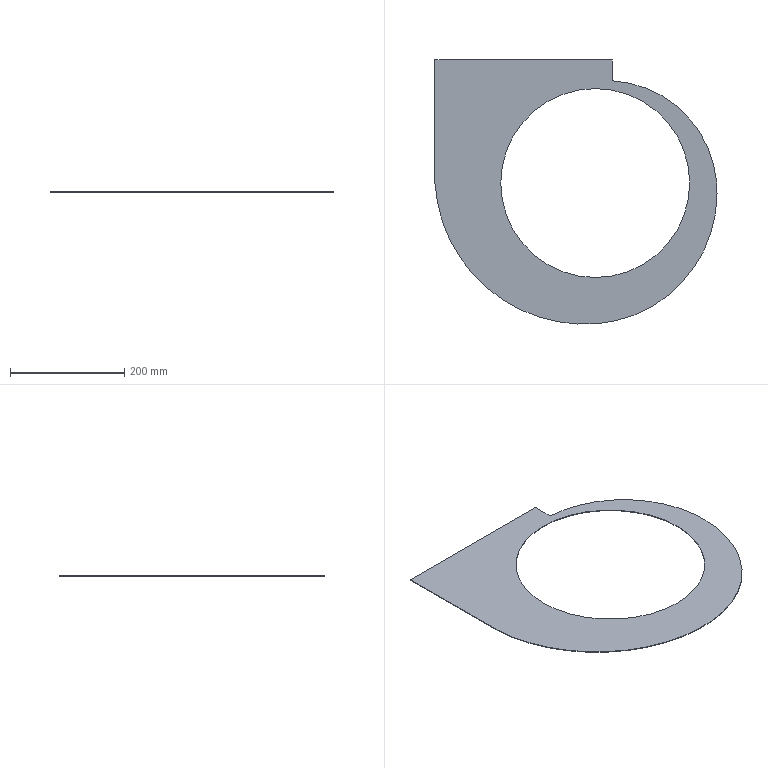Part | STEP file | HESS-408-70-15W-N-7-inner liner turbine panel | 1 solid | 11 faces | box 492.743 x 461.634 x 1 mm | volume 101400 mm3 | cylinder 6 | plane 5 | commonest cylinder face diameters 330 x2 456.243 x2 387.951 x1 524.472 x1
STEP:
#1=CARTESIAN_POINT('',(0.,0.,0.));
#2=DIRECTION('',(0.,0.,1.));
#3=DIRECTION('',(1.,0.,0.));
#4=AXIS2_PLACEMENT_3D('',#1,#2,#3);
#5=CARTESIAN_POINT('',(2081.954,652.923,-1.));
#6=VERTEX_POINT('',#5);
#7=CARTESIAN_POINT('',(2291.02,880.247,-1.));
#8=VERTEX_POINT('',#7);
#9=CARTESIAN_POINT('',(2062.898,880.247,-1.));
#10=DIRECTION('',(0.,0.,1.));
#11=DIRECTION('',(1.,0.,0.));
#12=AXIS2_PLACEMENT_3D('',#9,#10,#11);
#13=CIRCLE('',#12,228.121);
#14=CARTESIAN_POINT('',(2062.898,880.247,-1.));
#15=DIRECTION('',(0.,0.,1.));
#16=DIRECTION('',(1.,0.,0.));
#17=AXIS2_PLACEMENT_3D('',#14,#15,#16);
#18=CYLINDRICAL_SURFACE('',#17,228.121);
#19=CARTESIAN_POINT('',(0.,0.));
#20=DIRECTION('',(1.,0.));
#21=VECTOR('',#20,1.);
#22=LINE('',#19,#21);
#23=(GEOMETRIC_REPRESENTATION_CONTEXT(2)PARAMETRIC_REPRESENTATION_CONTEXT()REPRESENTATION_CONTEXT('',''));
#24=DEFINITIONAL_REPRESENTATION('',(#22),#23);
#25=PCURVE('',#18,#24);
#26=CARTESIAN_POINT('',(2062.898,880.247,-1.));
#27=DIRECTION('',(0.,0.,1.));
#28=DIRECTION('',(1.,0.,0.));
#29=AXIS2_PLACEMENT_3D('',#26,#27,#28);
#30=PLANE('',#29);
#31=CARTESIAN_POINT('',(0.,0.));
#32=DIRECTION('',(1.,0.));
#33=AXIS2_PLACEMENT_2D('',#31,#32);
#34=CIRCLE('',#33,228.121);
#35=(GEOMETRIC_REPRESENTATION_CONTEXT(2)PARAMETRIC_REPRESENTATION_CONTEXT()REPRESENTATION_CONTEXT('',''));
#36=DEFINITIONAL_REPRESENTATION('',(#34),#35);
#37=PCURVE('',#30,#36);
#38=SURFACE_CURVE('',#13,(#25,#37),.PCURVE_S1.);
#39=EDGE_CURVE('',#6,#8,#38,.T.);
#40=ORIENTED_EDGE('',*,*,#39,.T.);
#41=CARTESIAN_POINT('',(2291.02,880.247,0.));
#42=VERTEX_POINT('',#41);
#43=CARTESIAN_POINT('',(2291.02,880.247,-1.));
#44=DIRECTION('',(0.,0.,1.));
#45=VECTOR('',#44,1.);
#46=LINE('',#43,#45);
#47=CARTESIAN_POINT('',(6.283,0.));
#48=DIRECTION('',(0.,1.));
#49=VECTOR('',#48,1.);
#50=LINE('',#47,#49);
#51=(GEOMETRIC_REPRESENTATION_CONTEXT(2)PARAMETRIC_REPRESENTATION_CONTEXT()REPRESENTATION_CONTEXT('',''));
#52=DEFINITIONAL_REPRESENTATION('',(#50),#51);
#53=PCURVE('',#18,#52);
#54=CARTESIAN_POINT('',(2062.898,880.247,-1.));
#55=DIRECTION('',(0.,0.,1.));
#56=DIRECTION('',(1.,0.,0.));
#57=AXIS2_PLACEMENT_3D('',#54,#55,#56);
#58=CYLINDRICAL_SURFACE('',#57,228.121);
#59=CARTESIAN_POINT('',(0.,0.));
#60=DIRECTION('',(0.,1.));
#61=VECTOR('',#60,1.);
#62=LINE('',#59,#61);
#63=(GEOMETRIC_REPRESENTATION_CONTEXT(2)PARAMETRIC_REPRESENTATION_CONTEXT()REPRESENTATION_CONTEXT('',''));
#64=DEFINITIONAL_REPRESENTATION('',(#62),#63);
#65=PCURVE('',#58,#64);
#66=SURFACE_CURVE('',#46,(#53,#65),.PCURVE_S1.);
#67=EDGE_CURVE('',#8,#42,#66,.T.);
#68=ORIENTED_EDGE('',*,*,#67,.T.);
#69=CARTESIAN_POINT('',(2081.954,652.923,0.));
#70=VERTEX_POINT('',#69);
#71=CARTESIAN_POINT('',(2062.898,880.247,0.));
#72=DIRECTION('',(0.,0.,1.));
#73=DIRECTION('',(1.,0.,0.));
#74=AXIS2_PLACEMENT_3D('',#71,#72,#73);
#75=CIRCLE('',#74,228.121);
#76=CARTESIAN_POINT('',(0.,1.));
#77=DIRECTION('',(1.,0.));
#78=VECTOR('',#77,1.);
#79=LINE('',#76,#78);
#80=(GEOMETRIC_REPRESENTATION_CONTEXT(2)PARAMETRIC_REPRESENTATION_CONTEXT()REPRESENTATION_CONTEXT('',''));
#81=DEFINITIONAL_REPRESENTATION('',(#79),#80);
#82=PCURVE('',#18,#81);
#83=CARTESIAN_POINT('',(2062.898,880.247,0.));
#84=DIRECTION('',(0.,0.,1.));
#85=DIRECTION('',(1.,0.,0.));
#86=AXIS2_PLACEMENT_3D('',#83,#84,#85);
#87=PLANE('',#86);
#88=CARTESIAN_POINT('',(0.,0.));
#89=DIRECTION('',(1.,0.));
#90=AXIS2_PLACEMENT_2D('',#88,#89);
#91=CIRCLE('',#90,228.121);
#92=(GEOMETRIC_REPRESENTATION_CONTEXT(2)PARAMETRIC_REPRESENTATION_CONTEXT()REPRESENTATION_CONTEXT('',''));
#93=DEFINITIONAL_REPRESENTATION('',(#91),#92);
#94=PCURVE('',#87,#93);
#95=SURFACE_CURVE('',#75,(#82,#94),.PCURVE_S1.);
#96=EDGE_CURVE('',#70,#42,#95,.T.);
#97=ORIENTED_EDGE('',*,*,#96,.F.);
#98=CARTESIAN_POINT('',(2081.954,652.923,-1.));
#99=DIRECTION('',(0.,0.,1.));
#100=VECTOR('',#99,1.);
#101=LINE('',#98,#100);
#102=CARTESIAN_POINT('',(4.796,0.));
#103=DIRECTION('',(0.,1.));
#104=VECTOR('',#103,1.);
#105=LINE('',#102,#104);
#106=(GEOMETRIC_REPRESENTATION_CONTEXT(2)PARAMETRIC_REPRESENTATION_CONTEXT()REPRESENTATION_CONTEXT('',''));
#107=DEFINITIONAL_REPRESENTATION('',(#105),#106);
#108=PCURVE('',#18,#107);
#109=CARTESIAN_POINT('',(2060.048,914.242,-1.));
#110=DIRECTION('',(0.,0.,1.));
#111=DIRECTION('',(1.,0.,0.));
#112=AXIS2_PLACEMENT_3D('',#109,#110,#111);
#113=CYLINDRICAL_SURFACE('',#112,262.236);
#114=CARTESIAN_POINT('',(4.796,0.));
#115=DIRECTION('',(0.,1.));
#116=VECTOR('',#115,1.);
#117=LINE('',#114,#116);
#118=(GEOMETRIC_REPRESENTATION_CONTEXT(2)PARAMETRIC_REPRESENTATION_CONTEXT()REPRESENTATION_CONTEXT('',''));
#119=DEFINITIONAL_REPRESENTATION('',(#117),#118);
#120=PCURVE('',#113,#119);
#121=SURFACE_CURVE('',#101,(#108,#120),.PCURVE_S1.);
#122=EDGE_CURVE('',#6,#70,#121,.T.);
#123=ORIENTED_EDGE('',*,*,#122,.F.);
#124=EDGE_LOOP('',(#40,#68,#97,#123));
#125=FACE_BOUND('',#124,.T.);
#126=ADVANCED_FACE('',(#125),#18,.T.);
#127=CARTESIAN_POINT('',(2243.277,898.641,-1.));
#128=VERTEX_POINT('',#127);
#129=CARTESIAN_POINT('',(2243.277,898.641,0.));
#130=VERTEX_POINT('',#129);
#131=CARTESIAN_POINT('',(2243.277,898.641,-1.));
#132=DIRECTION('',(0.,0.,1.));
#133=VECTOR('',#132,1.);
#134=LINE('',#131,#133);
#135=CARTESIAN_POINT('',(2078.277,898.641,-1.));
#136=DIRECTION('',(0.,0.,1.));
#137=DIRECTION('',(1.,0.,0.));
#138=AXIS2_PLACEMENT_3D('',#135,#136,#137);
#139=CYLINDRICAL_SURFACE('',#138,165.);
#140=CARTESIAN_POINT('',(6.283,0.));
#141=DIRECTION('',(0.,1.));
#142=VECTOR('',#141,1.);
#143=LINE('',#140,#142);
#144=(GEOMETRIC_REPRESENTATION_CONTEXT(2)PARAMETRIC_REPRESENTATION_CONTEXT()REPRESENTATION_CONTEXT('',''));
#145=DEFINITIONAL_REPRESENTATION('',(#143),#144);
#146=PCURVE('',#139,#145);
#147=CARTESIAN_POINT('',(2078.277,898.641,-1.));
#148=DIRECTION('',(0.,0.,1.));
#149=DIRECTION('',(1.,0.,0.));
#150=AXIS2_PLACEMENT_3D('',#147,#148,#149);
#151=CYLINDRICAL_SURFACE('',#150,165.);
#152=CARTESIAN_POINT('',(0.,0.));
#153=DIRECTION('',(0.,1.));
#154=VECTOR('',#153,1.);
#155=LINE('',#152,#154);
#156=(GEOMETRIC_REPRESENTATION_CONTEXT(2)PARAMETRIC_REPRESENTATION_CONTEXT()REPRESENTATION_CONTEXT('',''));
#157=DEFINITIONAL_REPRESENTATION('',(#155),#156);
#158=PCURVE('',#151,#157);
#159=SURFACE_CURVE('',#134,(#146,#158),.PCURVE_S1.);
#160=EDGE_CURVE('',#128,#130,#159,.T.);
#161=ORIENTED_EDGE('',*,*,#160,.T.);
#162=CARTESIAN_POINT('',(1913.277,898.641,0.));
#163=VERTEX_POINT('',#162);
#164=CARTESIAN_POINT('',(2078.277,898.641,0.));
#165=DIRECTION('',(0.,0.,-1.));
#166=DIRECTION('',(1.,0.,0.));
#167=AXIS2_PLACEMENT_3D('',#164,#165,#166);
#168=CIRCLE('',#167,165.);
#169=CARTESIAN_POINT('',(6.283,1.));
#170=DIRECTION('',(-1.,0.));
#171=VECTOR('',#170,1.);
#172=LINE('',#169,#171);
#173=(GEOMETRIC_REPRESENTATION_CONTEXT(2)PARAMETRIC_REPRESENTATION_CONTEXT()REPRESENTATION_CONTEXT('',''));
#174=DEFINITIONAL_REPRESENTATION('',(#172),#173);
#175=PCURVE('',#139,#174);
#176=CARTESIAN_POINT('',(180.379,18.394));
#177=CARTESIAN_POINT('',(180.379,-267.395));
#178=CARTESIAN_POINT('',(-67.121,-124.5));
#179=CARTESIAN_POINT('',(-314.621,18.394));
#180=CARTESIAN_POINT('',(-67.121,161.288));
#181=CARTESIAN_POINT('',(180.379,304.182));
#182=CARTESIAN_POINT('',(180.379,18.394));
#183=(BOUNDED_CURVE()B_SPLINE_CURVE(2,(#176,#177,#178,#179,#180,#181,#182),.UNSPECIFIED.,.T.,.F.)B_SPLINE_CURVE_WITH_KNOTS((1,2,2,2,2,1),(-2.094,0.,2.094,4.189,6.283,8.378),.UNSPECIFIED.)CURVE()GEOMETRIC_REPRESENTATION_ITEM()RATIONAL_B_SPLINE_CURVE((1.,0.5,1.,0.5,1.,0.5,1.))REPRESENTATION_ITEM(''));
#184=(GEOMETRIC_REPRESENTATION_CONTEXT(2)PARAMETRIC_REPRESENTATION_CONTEXT()REPRESENTATION_CONTEXT('',''));
#185=DEFINITIONAL_REPRESENTATION('',(#183),#184);
#186=PCURVE('',#87,#185);
#187=SURFACE_CURVE('',#168,(#175,#186),.PCURVE_S1.);
#188=EDGE_CURVE('',#130,#163,#187,.T.);
#189=ORIENTED_EDGE('',*,*,#188,.T.);
#190=CARTESIAN_POINT('',(1913.277,898.641,-1.));
#191=VERTEX_POINT('',#190);
#192=CARTESIAN_POINT('',(1913.277,898.641,-1.));
#193=DIRECTION('',(0.,0.,1.));
#194=VECTOR('',#193,1.);
#195=LINE('',#192,#194);
#196=CARTESIAN_POINT('',(3.142,0.));
#197=DIRECTION('',(0.,1.));
#198=VECTOR('',#197,1.);
#199=LINE('',#196,#198);
#200=(GEOMETRIC_REPRESENTATION_CONTEXT(2)PARAMETRIC_REPRESENTATION_CONTEXT()REPRESENTATION_CONTEXT('',''));
#201=DEFINITIONAL_REPRESENTATION('',(#199),#200);
#202=PCURVE('',#139,#201);
#203=CARTESIAN_POINT('',(3.142,0.));
#204=DIRECTION('',(0.,1.));
#205=VECTOR('',#204,1.);
#206=LINE('',#203,#205);
#207=(GEOMETRIC_REPRESENTATION_CONTEXT(2)PARAMETRIC_REPRESENTATION_CONTEXT()REPRESENTATION_CONTEXT('',''));
#208=DEFINITIONAL_REPRESENTATION('',(#206),#207);
#209=PCURVE('',#151,#208);
#210=SURFACE_CURVE('',#195,(#202,#209),.PCURVE_S1.);
#211=EDGE_CURVE('',#191,#163,#210,.T.);
#212=ORIENTED_EDGE('',*,*,#211,.F.);
#213=CARTESIAN_POINT('',(2078.277,898.641,-1.));
#214=DIRECTION('',(0.,0.,1.));
#215=DIRECTION('',(1.,0.,0.));
#216=AXIS2_PLACEMENT_3D('',#213,#214,#215);
#217=CIRCLE('',#216,165.);
#218=CARTESIAN_POINT('',(0.,0.));
#219=DIRECTION('',(1.,0.));
#220=VECTOR('',#219,1.);
#221=LINE('',#218,#220);
#222=(GEOMETRIC_REPRESENTATION_CONTEXT(2)PARAMETRIC_REPRESENTATION_CONTEXT()REPRESENTATION_CONTEXT('',''));
#223=DEFINITIONAL_REPRESENTATION('',(#221),#222);
#224=PCURVE('',#139,#223);
#225=CARTESIAN_POINT('',(15.379,18.394));
#226=DIRECTION('',(1.,0.));
#227=AXIS2_PLACEMENT_2D('',#225,#226);
#228=CIRCLE('',#227,165.);
#229=(GEOMETRIC_REPRESENTATION_CONTEXT(2)PARAMETRIC_REPRESENTATION_CONTEXT()REPRESENTATION_CONTEXT('',''));
#230=DEFINITIONAL_REPRESENTATION('',(#228),#229);
#231=PCURVE('',#30,#230);
#232=SURFACE_CURVE('',#217,(#224,#231),.PCURVE_S1.);
#233=EDGE_CURVE('',#191,#128,#232,.T.);
#234=ORIENTED_EDGE('',*,*,#233,.T.);
#235=EDGE_LOOP('',(#161,#189,#212,#234));
#236=FACE_BOUND('',#235,.F.);
#237=ADVANCED_FACE('',(#236),#139,.F.);
#238=CARTESIAN_POINT('',(1798.277,1113.641,0.));
#239=VERTEX_POINT('',#238);
#240=CARTESIAN_POINT('',(1798.277,898.641,0.));
#241=VERTEX_POINT('',#240);
#242=CARTESIAN_POINT('',(1798.277,880.247,0.));
#243=DIRECTION('',(0.,-1.,0.));
#244=VECTOR('',#243,1.);
#245=LINE('',#242,#244);
#246=CARTESIAN_POINT('',(-264.621,0.));
#247=DIRECTION('',(0.,-1.));
#248=VECTOR('',#247,1.);
#249=LINE('',#246,#248);
#250=(GEOMETRIC_REPRESENTATION_CONTEXT(2)PARAMETRIC_REPRESENTATION_CONTEXT()REPRESENTATION_CONTEXT('',''));
#251=DEFINITIONAL_REPRESENTATION('',(#249),#250);
#252=PCURVE('',#87,#251);
#253=CARTESIAN_POINT('',(1798.277,898.641,-1.));
#254=DIRECTION('',(-1.,0.,0.));
#255=DIRECTION('',(0.,-1.,0.));
#256=AXIS2_PLACEMENT_3D('',#253,#254,#255);
#257=PLANE('',#256);
#258=CARTESIAN_POINT('',(18.394,1.));
#259=DIRECTION('',(1.,0.));
#260=VECTOR('',#259,1.);
#261=LINE('',#258,#260);
#262=(GEOMETRIC_REPRESENTATION_CONTEXT(2)PARAMETRIC_REPRESENTATION_CONTEXT()REPRESENTATION_CONTEXT('',''));
#263=DEFINITIONAL_REPRESENTATION('',(#261),#262);
#264=PCURVE('',#257,#263);
#265=SURFACE_CURVE('',#245,(#252,#264),.PCURVE_S1.);
#266=EDGE_CURVE('',#239,#241,#265,.T.);
#267=ORIENTED_EDGE('',*,*,#266,.T.);
#268=CARTESIAN_POINT('',(2060.048,914.242,0.));
#269=DIRECTION('',(0.,0.,1.));
#270=DIRECTION('',(1.,0.,0.));
#271=AXIS2_PLACEMENT_3D('',#268,#269,#270);
#272=CIRCLE('',#271,262.236);
#273=CARTESIAN_POINT('',(-2.85,33.996));
#274=DIRECTION('',(1.,0.));
#275=AXIS2_PLACEMENT_2D('',#273,#274);
#276=CIRCLE('',#275,262.236);
#277=(GEOMETRIC_REPRESENTATION_CONTEXT(2)PARAMETRIC_REPRESENTATION_CONTEXT()REPRESENTATION_CONTEXT('',''));
#278=DEFINITIONAL_REPRESENTATION('',(#276),#277);
#279=PCURVE('',#87,#278);
#280=CARTESIAN_POINT('',(0.,1.));
#281=DIRECTION('',(1.,0.));
#282=VECTOR('',#281,1.);
#283=LINE('',#280,#282);
#284=(GEOMETRIC_REPRESENTATION_CONTEXT(2)PARAMETRIC_REPRESENTATION_CONTEXT()REPRESENTATION_CONTEXT('',''));
#285=DEFINITIONAL_REPRESENTATION('',(#283),#284);
#286=PCURVE('',#113,#285);
#287=SURFACE_CURVE('',#272,(#279,#286),.PCURVE_S1.);
#288=EDGE_CURVE('',#241,#70,#287,.T.);
#289=ORIENTED_EDGE('',*,*,#288,.T.);
#290=ORIENTED_EDGE('',*,*,#96,.T.);
#291=CARTESIAN_POINT('',(2289.943,902.379,0.));
#292=VERTEX_POINT('',#291);
#293=CARTESIAN_POINT('',(2062.898,880.247,0.));
#294=DIRECTION('',(0.,0.,1.));
#295=DIRECTION('',(1.,0.,0.));
#296=AXIS2_PLACEMENT_3D('',#293,#294,#295);
#297=CIRCLE('',#296,228.121);
#298=CARTESIAN_POINT('',(0.,0.));
#299=DIRECTION('',(1.,0.));
#300=AXIS2_PLACEMENT_2D('',#298,#299);
#301=CIRCLE('',#300,228.121);
#302=(GEOMETRIC_REPRESENTATION_CONTEXT(2)PARAMETRIC_REPRESENTATION_CONTEXT()REPRESENTATION_CONTEXT('',''));
#303=DEFINITIONAL_REPRESENTATION('',(#301),#302);
#304=PCURVE('',#87,#303);
#305=CARTESIAN_POINT('',(0.,1.));
#306=DIRECTION('',(1.,0.));
#307=VECTOR('',#306,1.);
#308=LINE('',#305,#307);
#309=(GEOMETRIC_REPRESENTATION_CONTEXT(2)PARAMETRIC_REPRESENTATION_CONTEXT()REPRESENTATION_CONTEXT('',''));
#310=DEFINITIONAL_REPRESENTATION('',(#308),#309);
#311=PCURVE('',#58,#310);
#312=SURFACE_CURVE('',#297,(#304,#311),.PCURVE_S1.);
#313=EDGE_CURVE('',#42,#292,#312,.T.);
#314=ORIENTED_EDGE('',*,*,#313,.T.);
#315=CARTESIAN_POINT('',(2108.277,1077.2,0.));
#316=VERTEX_POINT('',#315);
#317=CARTESIAN_POINT('',(2096.883,883.56,0.));
#318=DIRECTION('',(0.,0.,1.));
#319=DIRECTION('',(1.,0.,0.));
#320=AXIS2_PLACEMENT_3D('',#317,#318,#319);
#321=CIRCLE('',#320,193.975);
#322=CARTESIAN_POINT('',(33.985,3.313));
#323=DIRECTION('',(1.,0.));
#324=AXIS2_PLACEMENT_2D('',#322,#323);
#325=CIRCLE('',#324,193.975);
#326=(GEOMETRIC_REPRESENTATION_CONTEXT(2)PARAMETRIC_REPRESENTATION_CONTEXT()REPRESENTATION_CONTEXT('',''));
#327=DEFINITIONAL_REPRESENTATION('',(#325),#326);
#328=PCURVE('',#87,#327);
#329=CARTESIAN_POINT('',(2096.883,883.56,-1.));
#330=DIRECTION('',(0.,0.,1.));
#331=DIRECTION('',(1.,0.,0.));
#332=AXIS2_PLACEMENT_3D('',#329,#330,#331);
#333=CYLINDRICAL_SURFACE('',#332,193.975);
#334=CARTESIAN_POINT('',(0.,1.));
#335=DIRECTION('',(1.,0.));
#336=VECTOR('',#335,1.);
#337=LINE('',#334,#336);
#338=(GEOMETRIC_REPRESENTATION_CONTEXT(2)PARAMETRIC_REPRESENTATION_CONTEXT()REPRESENTATION_CONTEXT('',''));
#339=DEFINITIONAL_REPRESENTATION('',(#337),#338);
#340=PCURVE('',#333,#339);
#341=SURFACE_CURVE('',#321,(#328,#340),.PCURVE_S1.);
#342=EDGE_CURVE('',#292,#316,#341,.T.);
#343=ORIENTED_EDGE('',*,*,#342,.T.);
#344=CARTESIAN_POINT('',(2108.277,1113.641,0.));
#345=VERTEX_POINT('',#344);
#346=CARTESIAN_POINT('',(2108.277,880.247,0.));
#347=DIRECTION('',(0.,1.,0.));
#348=VECTOR('',#347,1.);
#349=LINE('',#346,#348);
#350=CARTESIAN_POINT('',(45.379,0.));
#351=DIRECTION('',(0.,1.));
#352=VECTOR('',#351,1.);
#353=LINE('',#350,#352);
#354=(GEOMETRIC_REPRESENTATION_CONTEXT(2)PARAMETRIC_REPRESENTATION_CONTEXT()REPRESENTATION_CONTEXT('',''));
#355=DEFINITIONAL_REPRESENTATION('',(#353),#354);
#356=PCURVE('',#87,#355);
#357=CARTESIAN_POINT('',(2108.277,1113.641,-1.));
#358=DIRECTION('',(1.,0.,0.));
#359=DIRECTION('',(0.,0.,-1.));
#360=AXIS2_PLACEMENT_3D('',#357,#358,#359);
#361=PLANE('',#360);
#362=CARTESIAN_POINT('',(-1.,-233.394));
#363=DIRECTION('',(0.,1.));
#364=VECTOR('',#363,1.);
#365=LINE('',#362,#364);
#366=(GEOMETRIC_REPRESENTATION_CONTEXT(2)PARAMETRIC_REPRESENTATION_CONTEXT()REPRESENTATION_CONTEXT('',''));
#367=DEFINITIONAL_REPRESENTATION('',(#365),#366);
#368=PCURVE('',#361,#367);
#369=SURFACE_CURVE('',#349,(#356,#368),.PCURVE_S1.);
#370=EDGE_CURVE('',#316,#345,#369,.T.);
#371=ORIENTED_EDGE('',*,*,#370,.T.);
#372=CARTESIAN_POINT('',(2062.898,1113.641,0.));
#373=DIRECTION('',(-1.,0.,0.));
#374=VECTOR('',#373,1.);
#375=LINE('',#372,#374);
#376=CARTESIAN_POINT('',(0.,233.394));
#377=DIRECTION('',(-1.,0.));
#378=VECTOR('',#377,1.);
#379=LINE('',#376,#378);
#380=(GEOMETRIC_REPRESENTATION_CONTEXT(2)PARAMETRIC_REPRESENTATION_CONTEXT()REPRESENTATION_CONTEXT('',''));
#381=DEFINITIONAL_REPRESENTATION('',(#379),#380);
#382=PCURVE('',#87,#381);
#383=CARTESIAN_POINT('',(2108.277,1113.641,-1.));
#384=DIRECTION('',(0.,1.,0.));
#385=DIRECTION('',(0.,0.,1.));
#386=AXIS2_PLACEMENT_3D('',#383,#384,#385);
#387=PLANE('',#386);
#388=CARTESIAN_POINT('',(1.,-45.379));
#389=DIRECTION('',(0.,-1.));
#390=VECTOR('',#389,1.);
#391=LINE('',#388,#390);
#392=(GEOMETRIC_REPRESENTATION_CONTEXT(2)PARAMETRIC_REPRESENTATION_CONTEXT()REPRESENTATION_CONTEXT('',''));
#393=DEFINITIONAL_REPRESENTATION('',(#391),#392);
#394=PCURVE('',#387,#393);
#395=SURFACE_CURVE('',#375,(#382,#394),.PCURVE_S1.);
#396=EDGE_CURVE('',#345,#239,#395,.T.);
#397=ORIENTED_EDGE('',*,*,#396,.T.);
#398=EDGE_LOOP('',(#267,#289,#290,#314,#343,#371,#397));
#399=FACE_BOUND('',#398,.T.);
#400=ORIENTED_EDGE('',*,*,#188,.T.);
#401=CARTESIAN_POINT('',(2078.277,898.641,0.));
#402=DIRECTION('',(0.,0.,-1.));
#403=DIRECTION('',(1.,0.,0.));
#404=AXIS2_PLACEMENT_3D('',#401,#402,#403);
#405=CIRCLE('',#404,165.);
#406=CARTESIAN_POINT('',(180.379,18.394));
#407=CARTESIAN_POINT('',(180.379,-267.395));
#408=CARTESIAN_POINT('',(-67.121,-124.5));
#409=CARTESIAN_POINT('',(-314.621,18.394));
#410=CARTESIAN_POINT('',(-67.121,161.288));
#411=CARTESIAN_POINT('',(180.379,304.182));
#412=CARTESIAN_POINT('',(180.379,18.394));
#413=(BOUNDED_CURVE()B_SPLINE_CURVE(2,(#406,#407,#408,#409,#410,#411,#412),.UNSPECIFIED.,.T.,.F.)B_SPLINE_CURVE_WITH_KNOTS((1,2,2,2,2,1),(-2.094,0.,2.094,4.189,6.283,8.378),.UNSPECIFIED.)CURVE()GEOMETRIC_REPRESENTATION_ITEM()RATIONAL_B_SPLINE_CURVE((1.,0.5,1.,0.5,1.,0.5,1.))REPRESENTATION_ITEM(''));
#414=(GEOMETRIC_REPRESENTATION_CONTEXT(2)PARAMETRIC_REPRESENTATION_CONTEXT()REPRESENTATION_CONTEXT('',''));
#415=DEFINITIONAL_REPRESENTATION('',(#413),#414);
#416=PCURVE('',#87,#415);
#417=CARTESIAN_POINT('',(6.283,1.));
#418=DIRECTION('',(-1.,0.));
#419=VECTOR('',#418,1.);
#420=LINE('',#417,#419);
#421=(GEOMETRIC_REPRESENTATION_CONTEXT(2)PARAMETRIC_REPRESENTATION_CONTEXT()REPRESENTATION_CONTEXT('',''));
#422=DEFINITIONAL_REPRESENTATION('',(#420),#421);
#423=PCURVE('',#151,#422);
#424=SURFACE_CURVE('',#405,(#416,#423),.PCURVE_S1.);
#425=EDGE_CURVE('',#163,#130,#424,.T.);
#426=ORIENTED_EDGE('',*,*,#425,.T.);
#427=EDGE_LOOP('',(#400,#426));
#428=FACE_BOUND('',#427,.T.);
#429=ADVANCED_FACE('',(#399,#428),#87,.T.);
#430=CARTESIAN_POINT('',(1798.277,898.641,-1.));
#431=VERTEX_POINT('',#430);
#432=CARTESIAN_POINT('',(2060.048,914.242,-1.));
#433=DIRECTION('',(0.,0.,1.));
#434=DIRECTION('',(1.,0.,0.));
#435=AXIS2_PLACEMENT_3D('',#432,#433,#434);
#436=CIRCLE('',#435,262.236);
#437=CARTESIAN_POINT('',(0.,0.));
#438=DIRECTION('',(1.,0.));
#439=VECTOR('',#438,1.);
#440=LINE('',#437,#439);
#441=(GEOMETRIC_REPRESENTATION_CONTEXT(2)PARAMETRIC_REPRESENTATION_CONTEXT()REPRESENTATION_CONTEXT('',''));
#442=DEFINITIONAL_REPRESENTATION('',(#440),#441);
#443=PCURVE('',#113,#442);
#444=CARTESIAN_POINT('',(-2.85,33.996));
#445=DIRECTION('',(1.,0.));
#446=AXIS2_PLACEMENT_2D('',#444,#445);
#447=CIRCLE('',#446,262.236);
#448=(GEOMETRIC_REPRESENTATION_CONTEXT(2)PARAMETRIC_REPRESENTATION_CONTEXT()REPRESENTATION_CONTEXT('',''));
#449=DEFINITIONAL_REPRESENTATION('',(#447),#448);
#450=PCURVE('',#30,#449);
#451=SURFACE_CURVE('',#436,(#443,#450),.PCURVE_S1.);
#452=EDGE_CURVE('',#431,#6,#451,.T.);
#453=ORIENTED_EDGE('',*,*,#452,.T.);
#454=ORIENTED_EDGE('',*,*,#122,.T.);
#455=ORIENTED_EDGE('',*,*,#288,.F.);
#456=CARTESIAN_POINT('',(1798.277,898.641,-1.));
#457=DIRECTION('',(0.,0.,-1.));
#458=VECTOR('',#457,1.);
#459=LINE('',#456,#458);
#460=CARTESIAN_POINT('',(3.201,0.));
#461=DIRECTION('',(0.,-1.));
#462=VECTOR('',#461,1.);
#463=LINE('',#460,#462);
#464=(GEOMETRIC_REPRESENTATION_CONTEXT(2)PARAMETRIC_REPRESENTATION_CONTEXT()REPRESENTATION_CONTEXT('',''));
#465=DEFINITIONAL_REPRESENTATION('',(#463),#464);
#466=PCURVE('',#113,#465);
#467=CARTESIAN_POINT('',(0.,0.));
#468=DIRECTION('',(0.,-1.));
#469=VECTOR('',#468,1.);
#470=LINE('',#467,#469);
#471=(GEOMETRIC_REPRESENTATION_CONTEXT(2)PARAMETRIC_REPRESENTATION_CONTEXT()REPRESENTATION_CONTEXT('',''));
#472=DEFINITIONAL_REPRESENTATION('',(#470),#471);
#473=PCURVE('',#257,#472);
#474=SURFACE_CURVE('',#459,(#466,#473),.PCURVE_S1.);
#475=EDGE_CURVE('',#241,#431,#474,.T.);
#476=ORIENTED_EDGE('',*,*,#475,.T.);
#477=EDGE_LOOP('',(#453,#454,#455,#476));
#478=FACE_BOUND('',#477,.T.);
#479=ADVANCED_FACE('',(#478),#113,.T.);
#480=CARTESIAN_POINT('',(1798.277,1113.641,-1.));
#481=VERTEX_POINT('',#480);
#482=CARTESIAN_POINT('',(1798.277,898.641,-1.));
#483=DIRECTION('',(0.,-1.,0.));
#484=VECTOR('',#483,1.);
#485=LINE('',#482,#484);
#486=CARTESIAN_POINT('',(0.,0.));
#487=DIRECTION('',(1.,0.));
#488=VECTOR('',#487,1.);
#489=LINE('',#486,#488);
#490=(GEOMETRIC_REPRESENTATION_CONTEXT(2)PARAMETRIC_REPRESENTATION_CONTEXT()REPRESENTATION_CONTEXT('',''));
#491=DEFINITIONAL_REPRESENTATION('',(#489),#490);
#492=PCURVE('',#257,#491);
#493=CARTESIAN_POINT('',(-264.621,18.394));
#494=DIRECTION('',(0.,-1.));
#495=VECTOR('',#494,1.);
#496=LINE('',#493,#495);
#497=(GEOMETRIC_REPRESENTATION_CONTEXT(2)PARAMETRIC_REPRESENTATION_CONTEXT()REPRESENTATION_CONTEXT('',''));
#498=DEFINITIONAL_REPRESENTATION('',(#496),#497);
#499=PCURVE('',#30,#498);
#500=SURFACE_CURVE('',#485,(#492,#499),.PCURVE_S1.);
#501=EDGE_CURVE('',#481,#431,#500,.T.);
#502=ORIENTED_EDGE('',*,*,#501,.T.);
#503=ORIENTED_EDGE('',*,*,#475,.F.);
#504=ORIENTED_EDGE('',*,*,#266,.F.);
#505=CARTESIAN_POINT('',(1798.277,1113.641,-1.));
#506=DIRECTION('',(0.,0.,-1.));
#507=VECTOR('',#506,1.);
#508=LINE('',#505,#507);
#509=CARTESIAN_POINT('',(-215.,0.));
#510=DIRECTION('',(0.,-1.));
#511=VECTOR('',#510,1.);
#512=LINE('',#509,#511);
#513=(GEOMETRIC_REPRESENTATION_CONTEXT(2)PARAMETRIC_REPRESENTATION_CONTEXT()REPRESENTATION_CONTEXT('',''));
#514=DEFINITIONAL_REPRESENTATION('',(#512),#513);
#515=PCURVE('',#257,#514);
#516=CARTESIAN_POINT('',(0.,-310.));
#517=DIRECTION('',(-1.,0.));
#518=VECTOR('',#517,1.);
#519=LINE('',#516,#518);
#520=(GEOMETRIC_REPRESENTATION_CONTEXT(2)PARAMETRIC_REPRESENTATION_CONTEXT()REPRESENTATION_CONTEXT('',''));
#521=DEFINITIONAL_REPRESENTATION('',(#519),#520);
#522=PCURVE('',#387,#521);
#523=SURFACE_CURVE('',#508,(#515,#522),.PCURVE_S1.);
#524=EDGE_CURVE('',#239,#481,#523,.T.);
#525=ORIENTED_EDGE('',*,*,#524,.T.);
#526=EDGE_LOOP('',(#502,#503,#504,#525));
#527=FACE_BOUND('',#526,.T.);
#528=ADVANCED_FACE('',(#527),#257,.T.);
#529=CARTESIAN_POINT('',(2108.277,1113.641,-1.));
#530=VERTEX_POINT('',#529);
#531=CARTESIAN_POINT('',(2108.277,1113.641,-1.));
#532=DIRECTION('',(-1.,0.,0.));
#533=VECTOR('',#532,1.);
#534=LINE('',#531,#533);
#535=CARTESIAN_POINT('',(0.,0.));
#536=DIRECTION('',(0.,-1.));
#537=VECTOR('',#536,1.);
#538=LINE('',#535,#537);
#539=(GEOMETRIC_REPRESENTATION_CONTEXT(2)PARAMETRIC_REPRESENTATION_CONTEXT()REPRESENTATION_CONTEXT('',''));
#540=DEFINITIONAL_REPRESENTATION('',(#538),#539);
#541=PCURVE('',#387,#540);
#542=CARTESIAN_POINT('',(45.379,233.394));
#543=DIRECTION('',(-1.,0.));
#544=VECTOR('',#543,1.);
#545=LINE('',#542,#544);
#546=(GEOMETRIC_REPRESENTATION_CONTEXT(2)PARAMETRIC_REPRESENTATION_CONTEXT()REPRESENTATION_CONTEXT('',''));
#547=DEFINITIONAL_REPRESENTATION('',(#545),#546);
#548=PCURVE('',#30,#547);
#549=SURFACE_CURVE('',#534,(#541,#548),.PCURVE_S1.);
#550=EDGE_CURVE('',#530,#481,#549,.T.);
#551=ORIENTED_EDGE('',*,*,#550,.T.);
#552=ORIENTED_EDGE('',*,*,#524,.F.);
#553=ORIENTED_EDGE('',*,*,#396,.F.);
#554=CARTESIAN_POINT('',(2108.277,1113.641,-1.));
#555=DIRECTION('',(0.,0.,-1.));
#556=VECTOR('',#555,1.);
#557=LINE('',#554,#556);
#558=CARTESIAN_POINT('',(0.,0.));
#559=DIRECTION('',(-1.,0.));
#560=VECTOR('',#559,1.);
#561=LINE('',#558,#560);
#562=(GEOMETRIC_REPRESENTATION_CONTEXT(2)PARAMETRIC_REPRESENTATION_CONTEXT()REPRESENTATION_CONTEXT('',''));
#563=DEFINITIONAL_REPRESENTATION('',(#561),#562);
#564=PCURVE('',#387,#563);
#565=CARTESIAN_POINT('',(0.,0.));
#566=DIRECTION('',(1.,0.));
#567=VECTOR('',#566,1.);
#568=LINE('',#565,#567);
#569=(GEOMETRIC_REPRESENTATION_CONTEXT(2)PARAMETRIC_REPRESENTATION_CONTEXT()REPRESENTATION_CONTEXT('',''));
#570=DEFINITIONAL_REPRESENTATION('',(#568),#569);
#571=PCURVE('',#361,#570);
#572=SURFACE_CURVE('',#557,(#564,#571),.PCURVE_S1.);
#573=EDGE_CURVE('',#345,#530,#572,.T.);
#574=ORIENTED_EDGE('',*,*,#573,.T.);
#575=EDGE_LOOP('',(#551,#552,#553,#574));
#576=FACE_BOUND('',#575,.T.);
#577=ADVANCED_FACE('',(#576),#387,.T.);
#578=CARTESIAN_POINT('',(2108.277,1077.2,-1.));
#579=VERTEX_POINT('',#578);
#580=CARTESIAN_POINT('',(2108.277,1113.641,-1.));
#581=DIRECTION('',(0.,1.,0.));
#582=VECTOR('',#581,1.);
#583=LINE('',#580,#582);
#584=CARTESIAN_POINT('',(0.,0.));
#585=DIRECTION('',(0.,1.));
#586=VECTOR('',#585,1.);
#587=LINE('',#584,#586);
#588=(GEOMETRIC_REPRESENTATION_CONTEXT(2)PARAMETRIC_REPRESENTATION_CONTEXT()REPRESENTATION_CONTEXT('',''));
#589=DEFINITIONAL_REPRESENTATION('',(#587),#588);
#590=PCURVE('',#361,#589);
#591=CARTESIAN_POINT('',(45.379,233.394));
#592=DIRECTION('',(0.,1.));
#593=VECTOR('',#592,1.);
#594=LINE('',#591,#593);
#595=(GEOMETRIC_REPRESENTATION_CONTEXT(2)PARAMETRIC_REPRESENTATION_CONTEXT()REPRESENTATION_CONTEXT('',''));
#596=DEFINITIONAL_REPRESENTATION('',(#594),#595);
#597=PCURVE('',#30,#596);
#598=SURFACE_CURVE('',#583,(#590,#597),.PCURVE_S1.);
#599=EDGE_CURVE('',#579,#530,#598,.T.);
#600=ORIENTED_EDGE('',*,*,#599,.T.);
#601=ORIENTED_EDGE('',*,*,#573,.F.);
#602=ORIENTED_EDGE('',*,*,#370,.F.);
#603=CARTESIAN_POINT('',(2108.277,1077.2,-1.));
#604=DIRECTION('',(0.,0.,-1.));
#605=VECTOR('',#604,1.);
#606=LINE('',#603,#605);
#607=CARTESIAN_POINT('',(0.,-36.44));
#608=DIRECTION('',(1.,0.));
#609=VECTOR('',#608,1.);
#610=LINE('',#607,#609);
#611=(GEOMETRIC_REPRESENTATION_CONTEXT(2)PARAMETRIC_REPRESENTATION_CONTEXT()REPRESENTATION_CONTEXT('',''));
#612=DEFINITIONAL_REPRESENTATION('',(#610),#611);
#613=PCURVE('',#361,#612);
#614=CARTESIAN_POINT('',(1.512,0.));
#615=DIRECTION('',(0.,-1.));
#616=VECTOR('',#615,1.);
#617=LINE('',#614,#616);
#618=(GEOMETRIC_REPRESENTATION_CONTEXT(2)PARAMETRIC_REPRESENTATION_CONTEXT()REPRESENTATION_CONTEXT('',''));
#619=DEFINITIONAL_REPRESENTATION('',(#617),#618);
#620=PCURVE('',#333,#619);
#621=SURFACE_CURVE('',#606,(#613,#620),.PCURVE_S1.);
#622=EDGE_CURVE('',#316,#579,#621,.T.);
#623=ORIENTED_EDGE('',*,*,#622,.T.);
#624=EDGE_LOOP('',(#600,#601,#602,#623));
#625=FACE_BOUND('',#624,.T.);
#626=ADVANCED_FACE('',(#625),#361,.T.);
#627=CARTESIAN_POINT('',(2289.943,902.379,-1.));
#628=VERTEX_POINT('',#627);
#629=CARTESIAN_POINT('',(2096.883,883.56,-1.));
#630=DIRECTION('',(0.,0.,1.));
#631=DIRECTION('',(1.,0.,0.));
#632=AXIS2_PLACEMENT_3D('',#629,#630,#631);
#633=CIRCLE('',#632,193.975);
#634=CARTESIAN_POINT('',(0.,0.));
#635=DIRECTION('',(1.,0.));
#636=VECTOR('',#635,1.);
#637=LINE('',#634,#636);
#638=(GEOMETRIC_REPRESENTATION_CONTEXT(2)PARAMETRIC_REPRESENTATION_CONTEXT()REPRESENTATION_CONTEXT('',''));
#639=DEFINITIONAL_REPRESENTATION('',(#637),#638);
#640=PCURVE('',#333,#639);
#641=CARTESIAN_POINT('',(33.985,3.313));
#642=DIRECTION('',(1.,0.));
#643=AXIS2_PLACEMENT_2D('',#641,#642);
#644=CIRCLE('',#643,193.975);
#645=(GEOMETRIC_REPRESENTATION_CONTEXT(2)PARAMETRIC_REPRESENTATION_CONTEXT()REPRESENTATION_CONTEXT('',''));
#646=DEFINITIONAL_REPRESENTATION('',(#644),#645);
#647=PCURVE('',#30,#646);
#648=SURFACE_CURVE('',#633,(#640,#647),.PCURVE_S1.);
#649=EDGE_CURVE('',#628,#579,#648,.T.);
#650=ORIENTED_EDGE('',*,*,#649,.T.);
#651=ORIENTED_EDGE('',*,*,#622,.F.);
#652=ORIENTED_EDGE('',*,*,#342,.F.);
#653=CARTESIAN_POINT('',(2289.943,902.379,-1.));
#654=DIRECTION('',(0.,0.,-1.));
#655=VECTOR('',#654,1.);
#656=LINE('',#653,#655);
#657=CARTESIAN_POINT('',(0.09717,0.));
#658=DIRECTION('',(0.,-1.));
#659=VECTOR('',#658,1.);
#660=LINE('',#657,#659);
#661=(GEOMETRIC_REPRESENTATION_CONTEXT(2)PARAMETRIC_REPRESENTATION_CONTEXT()REPRESENTATION_CONTEXT('',''));
#662=DEFINITIONAL_REPRESENTATION('',(#660),#661);
#663=PCURVE('',#333,#662);
#664=CARTESIAN_POINT('',(0.09717,0.));
#665=DIRECTION('',(0.,-1.));
#666=VECTOR('',#665,1.);
#667=LINE('',#664,#666);
#668=(GEOMETRIC_REPRESENTATION_CONTEXT(2)PARAMETRIC_REPRESENTATION_CONTEXT()REPRESENTATION_CONTEXT('',''));
#669=DEFINITIONAL_REPRESENTATION('',(#667),#668);
#670=PCURVE('',#58,#669);
#671=SURFACE_CURVE('',#656,(#663,#670),.PCURVE_S1.);
#672=EDGE_CURVE('',#292,#628,#671,.T.);
#673=ORIENTED_EDGE('',*,*,#672,.T.);
#674=EDGE_LOOP('',(#650,#651,#652,#673));
#675=FACE_BOUND('',#674,.T.);
#676=ADVANCED_FACE('',(#675),#333,.T.);
#677=ORIENTED_EDGE('',*,*,#67,.F.);
#678=CARTESIAN_POINT('',(2062.898,880.247,-1.));
#679=DIRECTION('',(0.,0.,1.));
#680=DIRECTION('',(1.,0.,0.));
#681=AXIS2_PLACEMENT_3D('',#678,#679,#680);
#682=CIRCLE('',#681,228.121);
#683=CARTESIAN_POINT('',(0.,0.));
#684=DIRECTION('',(1.,0.));
#685=VECTOR('',#684,1.);
#686=LINE('',#683,#685);
#687=(GEOMETRIC_REPRESENTATION_CONTEXT(2)PARAMETRIC_REPRESENTATION_CONTEXT()REPRESENTATION_CONTEXT('',''));
#688=DEFINITIONAL_REPRESENTATION('',(#686),#687);
#689=PCURVE('',#58,#688);
#690=CARTESIAN_POINT('',(0.,0.));
#691=DIRECTION('',(1.,0.));
#692=AXIS2_PLACEMENT_2D('',#690,#691);
#693=CIRCLE('',#692,228.121);
#694=(GEOMETRIC_REPRESENTATION_CONTEXT(2)PARAMETRIC_REPRESENTATION_CONTEXT()REPRESENTATION_CONTEXT('',''));
#695=DEFINITIONAL_REPRESENTATION('',(#693),#694);
#696=PCURVE('',#30,#695);
#697=SURFACE_CURVE('',#682,(#689,#696),.PCURVE_S1.);
#698=EDGE_CURVE('',#8,#628,#697,.T.);
#699=ORIENTED_EDGE('',*,*,#698,.T.);
#700=ORIENTED_EDGE('',*,*,#672,.F.);
#701=ORIENTED_EDGE('',*,*,#313,.F.);
#702=EDGE_LOOP('',(#677,#699,#700,#701));
#703=FACE_BOUND('',#702,.T.);
#704=ADVANCED_FACE('',(#703),#58,.T.);
#705=ORIENTED_EDGE('',*,*,#425,.T.);
#706=ORIENTED_EDGE('',*,*,#160,.F.);
#707=CARTESIAN_POINT('',(2078.277,898.641,-1.));
#708=DIRECTION('',(0.,0.,1.));
#709=DIRECTION('',(1.,0.,0.));
#710=AXIS2_PLACEMENT_3D('',#707,#708,#709);
#711=CIRCLE('',#710,165.);
#712=CARTESIAN_POINT('',(0.,0.));
#713=DIRECTION('',(1.,0.));
#714=VECTOR('',#713,1.);
#715=LINE('',#712,#714);
#716=(GEOMETRIC_REPRESENTATION_CONTEXT(2)PARAMETRIC_REPRESENTATION_CONTEXT()REPRESENTATION_CONTEXT('',''));
#717=DEFINITIONAL_REPRESENTATION('',(#715),#716);
#718=PCURVE('',#151,#717);
#719=CARTESIAN_POINT('',(15.379,18.394));
#720=DIRECTION('',(1.,0.));
#721=AXIS2_PLACEMENT_2D('',#719,#720);
#722=CIRCLE('',#721,165.);
#723=(GEOMETRIC_REPRESENTATION_CONTEXT(2)PARAMETRIC_REPRESENTATION_CONTEXT()REPRESENTATION_CONTEXT('',''));
#724=DEFINITIONAL_REPRESENTATION('',(#722),#723);
#725=PCURVE('',#30,#724);
#726=SURFACE_CURVE('',#711,(#718,#725),.PCURVE_S1.);
#727=EDGE_CURVE('',#128,#191,#726,.T.);
#728=ORIENTED_EDGE('',*,*,#727,.T.);
#729=ORIENTED_EDGE('',*,*,#211,.T.);
#730=EDGE_LOOP('',(#705,#706,#728,#729));
#731=FACE_BOUND('',#730,.F.);
#732=ADVANCED_FACE('',(#731),#151,.F.);
#733=ORIENTED_EDGE('',*,*,#452,.F.);
#734=ORIENTED_EDGE('',*,*,#501,.F.);
#735=ORIENTED_EDGE('',*,*,#550,.F.);
#736=ORIENTED_EDGE('',*,*,#599,.F.);
#737=ORIENTED_EDGE('',*,*,#649,.F.);
#738=ORIENTED_EDGE('',*,*,#698,.F.);
#739=ORIENTED_EDGE('',*,*,#39,.F.);
#740=EDGE_LOOP('',(#733,#734,#735,#736,#737,#738,#739));
#741=FACE_BOUND('',#740,.T.);
#742=ORIENTED_EDGE('',*,*,#727,.T.);
#743=ORIENTED_EDGE('',*,*,#233,.T.);
#744=EDGE_LOOP('',(#742,#743));
#745=FACE_BOUND('',#744,.T.);
#746=ADVANCED_FACE('',(#741,#745),#30,.F.);
#747=CLOSED_SHELL('',(#126,#237,#429,#479,#528,#577,#626,#676,#704,#732,#746));
#748=MANIFOLD_SOLID_BREP('',#747);
#749=(LENGTH_UNIT()NAMED_UNIT(*)SI_UNIT(.MILLI.,.METRE.));
#750=UNCERTAINTY_MEASURE_WITH_UNIT(LENGTH_MEASURE(0.0000001),#749,'','');
#751=(NAMED_UNIT(*)PLANE_ANGLE_UNIT()SI_UNIT($,.RADIAN.));
#752=(NAMED_UNIT(*)SI_UNIT($,.STERADIAN.)SOLID_ANGLE_UNIT());
#753=(GEOMETRIC_REPRESENTATION_CONTEXT(3)GLOBAL_UNCERTAINTY_ASSIGNED_CONTEXT((#750))GLOBAL_UNIT_ASSIGNED_CONTEXT((#749,#751,#752))REPRESENTATION_CONTEXT('',''));
#754=ADVANCED_BREP_SHAPE_REPRESENTATION('',(#4,#748),#753);